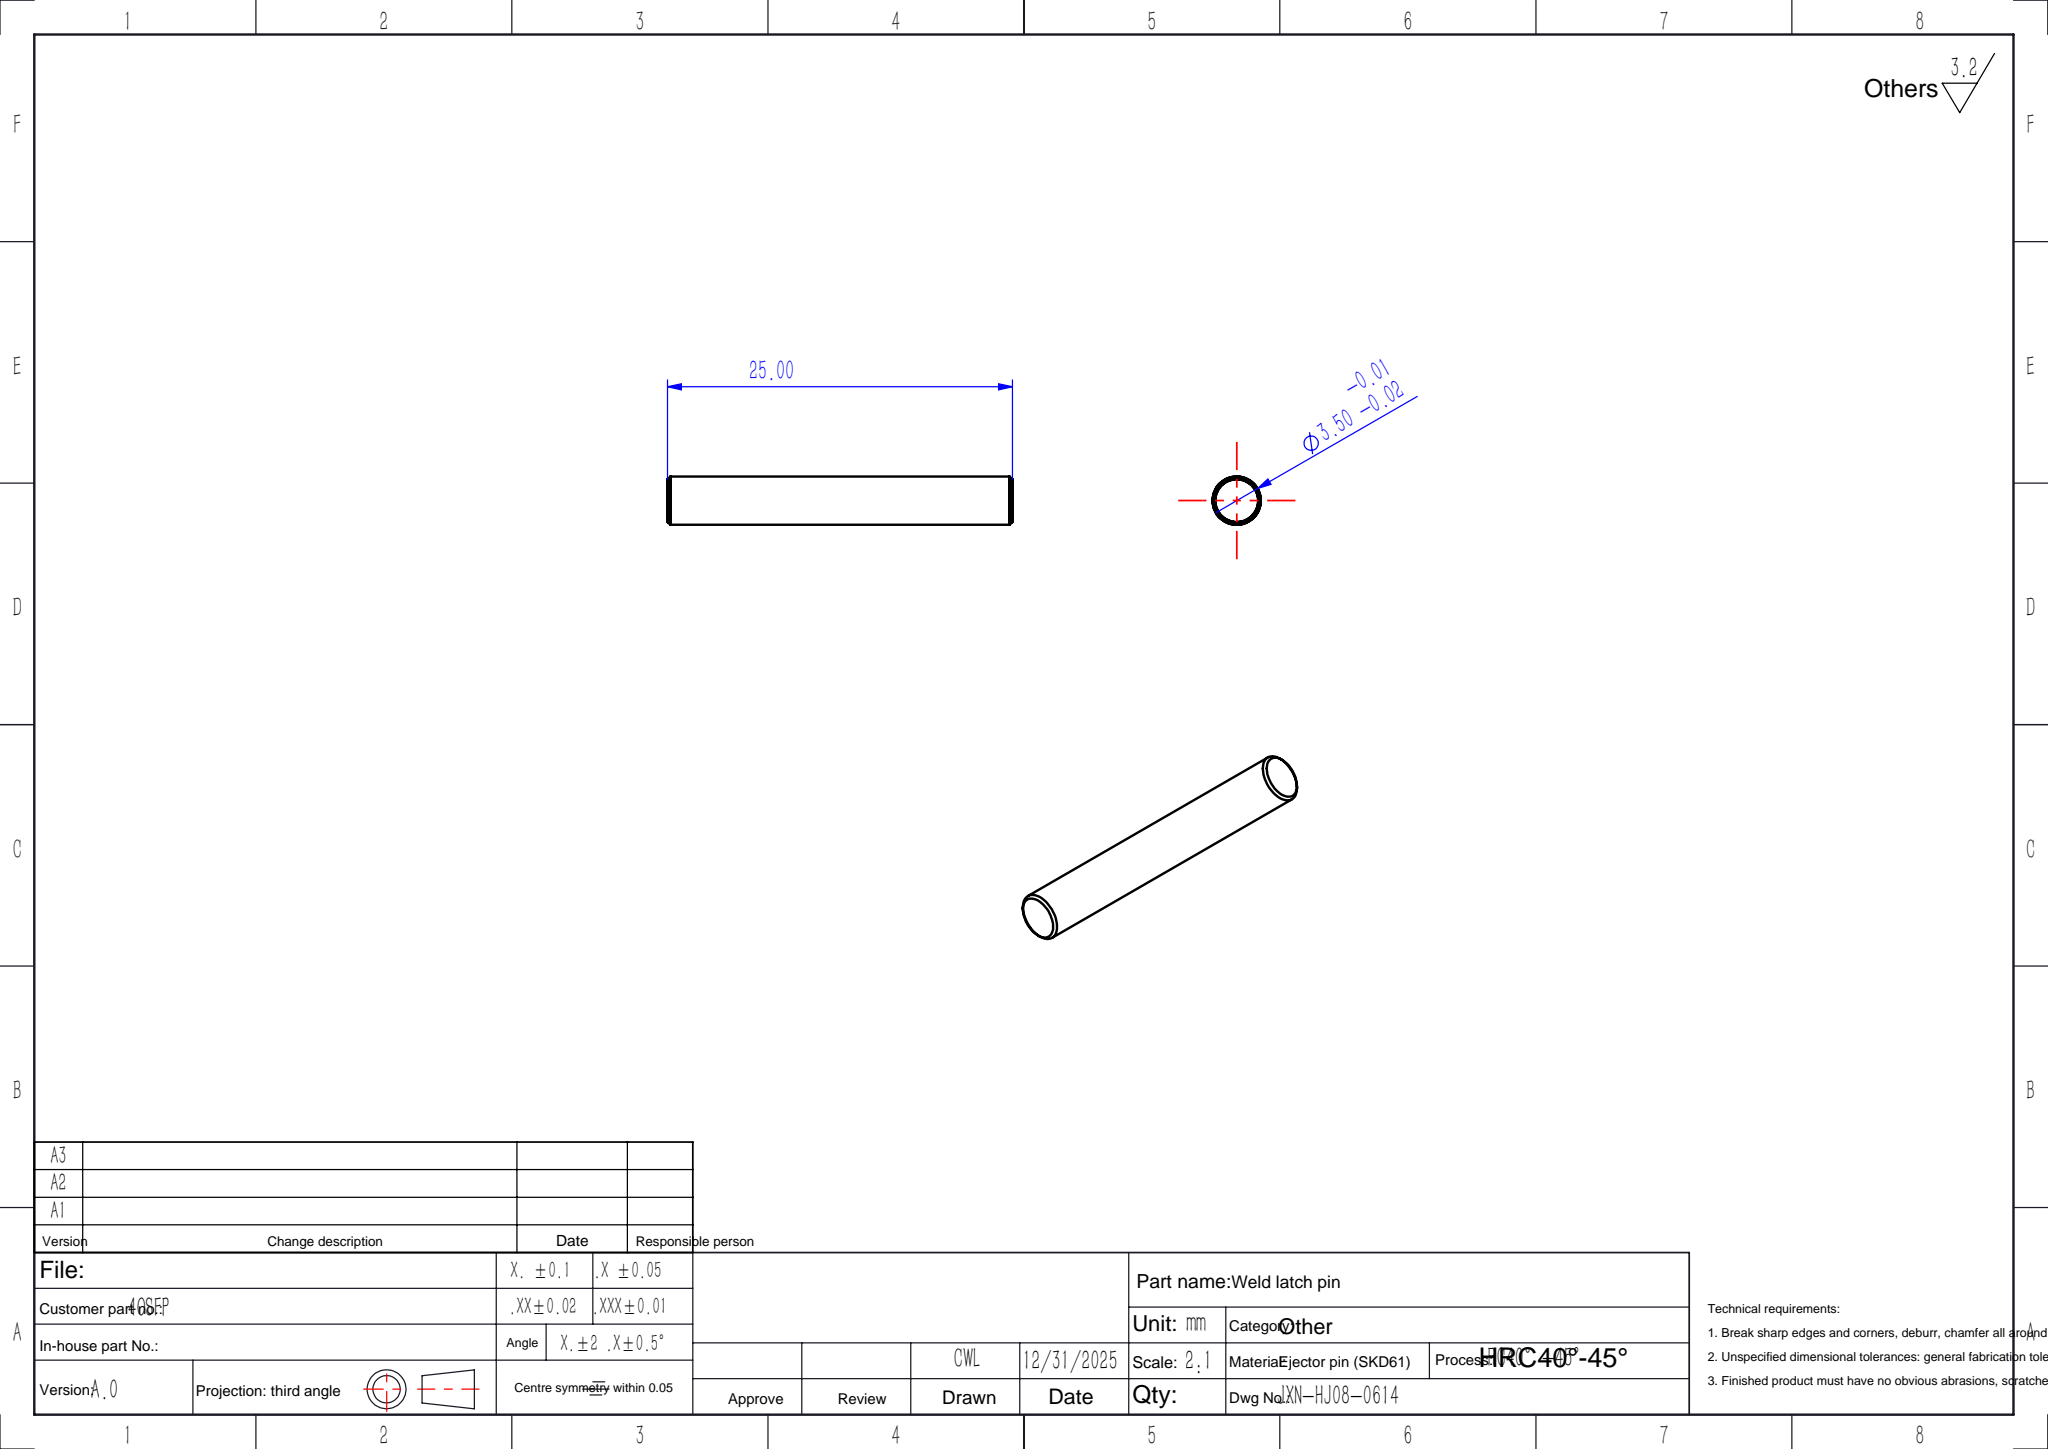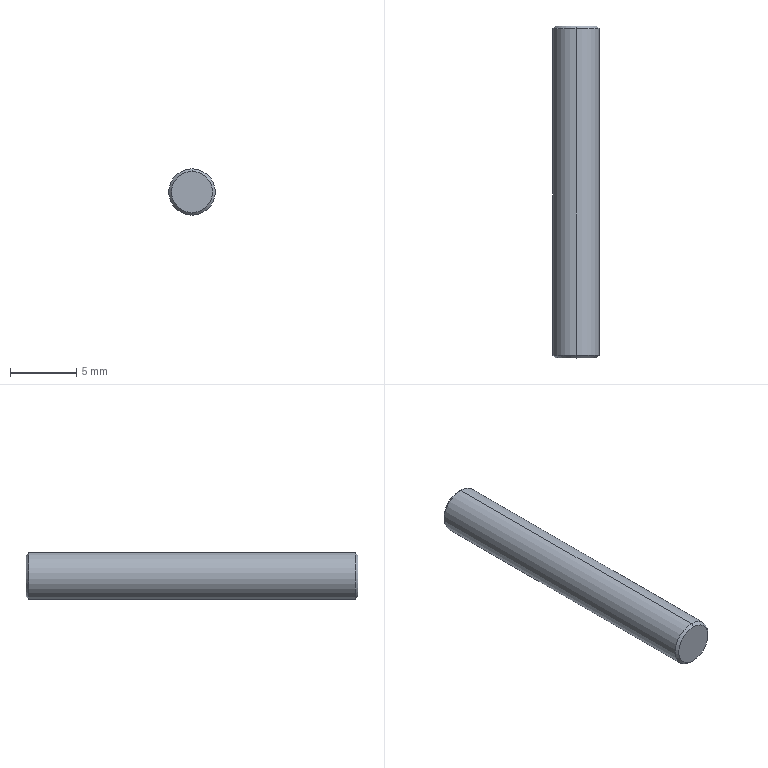Part | SolidWorks | features Chamfer 1, Extrusion 1 | 1 solid | 8 faces | box 3.5 x 25 x 3.5 mm | volume 240.105 mm3 | cone 4 | cylinder 2 | plane 2 | commonest cylinder face diameters 3.5 x2
STEP:
#1=CARTESIAN_POINT('',(0.,0.,-1.55));
#2=VERTEX_POINT('',#1);
#3=CARTESIAN_POINT('',(0.,0.,1.55));
#4=VERTEX_POINT('',#3);
#5=CARTESIAN_POINT('',(0.,0.,0.));
#6=DIRECTION('',(0.,-1.,0.));
#7=DIRECTION('',(0.,0.,1.));
#8=AXIS2_PLACEMENT_3D('',#5,#6,#7);
#9=CIRCLE('',#8,1.55);
#10=EDGE_CURVE('',#2,#4,#9,.T.);
#11=ORIENTED_EDGE('',*,*,#10,.F.);
#12=CARTESIAN_POINT('',(0.,0.2,-1.75));
#13=VERTEX_POINT('',#12);
#14=CARTESIAN_POINT('',(0.,0.2,-1.75));
#15=DIRECTION('',(0.,0.7071,-0.7071));
#16=VECTOR('',#15,1000.);
#17=LINE('',#14,#16);
#18=EDGE_CURVE('',#2,#13,#17,.T.);
#19=ORIENTED_EDGE('',*,*,#18,.T.);
#20=CARTESIAN_POINT('',(0.,0.2,1.75));
#21=VERTEX_POINT('',#20);
#22=CARTESIAN_POINT('',(0.,0.2,0.));
#23=DIRECTION('',(0.,1.,0.));
#24=DIRECTION('',(0.,0.,1.));
#25=AXIS2_PLACEMENT_3D('',#22,#23,#24);
#26=CIRCLE('',#25,1.75);
#27=EDGE_CURVE('',#21,#13,#26,.T.);
#28=ORIENTED_EDGE('',*,*,#27,.F.);
#29=CARTESIAN_POINT('',(0.,0.2,1.75));
#30=DIRECTION('',(0.,0.7071,0.7071));
#31=VECTOR('',#30,1000.);
#32=LINE('',#29,#31);
#33=EDGE_CURVE('',#4,#21,#32,.T.);
#34=ORIENTED_EDGE('',*,*,#33,.F.);
#35=EDGE_LOOP('',(#11,#19,#28,#34));
#36=FACE_OUTER_BOUND('',#35,.T.);
#37=CARTESIAN_POINT('',(0.,0.2,0.));
#38=DIRECTION('',(0.,1.,0.));
#39=DIRECTION('',(0.,0.,1.));
#40=AXIS2_PLACEMENT_3D('',#37,#38,#39);
#41=CONICAL_SURFACE('',#40,1.75,0.7854);
#42=ADVANCED_FACE('',(#36),#41,.T.);
#43=CARTESIAN_POINT('',(0.,25.,1.55));
#44=VERTEX_POINT('',#43);
#45=CARTESIAN_POINT('',(0.,25.,-1.55));
#46=VERTEX_POINT('',#45);
#47=CARTESIAN_POINT('',(0.,25.,0.));
#48=DIRECTION('',(0.,1.,0.));
#49=DIRECTION('',(0.,0.,1.));
#50=AXIS2_PLACEMENT_3D('',#47,#48,#49);
#51=CIRCLE('',#50,1.55);
#52=EDGE_CURVE('',#44,#46,#51,.T.);
#53=ORIENTED_EDGE('',*,*,#52,.F.);
#54=CARTESIAN_POINT('',(0.,24.8,1.75));
#55=VERTEX_POINT('',#54);
#56=CARTESIAN_POINT('',(0.,25.,1.55));
#57=DIRECTION('',(0.,-0.7071,0.7071));
#58=VECTOR('',#57,1000.);
#59=LINE('',#56,#58);
#60=EDGE_CURVE('',#44,#55,#59,.T.);
#61=ORIENTED_EDGE('',*,*,#60,.T.);
#62=CARTESIAN_POINT('',(0.,24.8,-1.75));
#63=VERTEX_POINT('',#62);
#64=CARTESIAN_POINT('',(0.,24.8,0.));
#65=DIRECTION('',(0.,-1.,0.));
#66=DIRECTION('',(0.,0.,1.));
#67=AXIS2_PLACEMENT_3D('',#64,#65,#66);
#68=CIRCLE('',#67,1.75);
#69=EDGE_CURVE('',#63,#55,#68,.T.);
#70=ORIENTED_EDGE('',*,*,#69,.F.);
#71=CARTESIAN_POINT('',(0.,25.,-1.55));
#72=DIRECTION('',(0.,-0.7071,-0.7071));
#73=VECTOR('',#72,1000.);
#74=LINE('',#71,#73);
#75=EDGE_CURVE('',#46,#63,#74,.T.);
#76=ORIENTED_EDGE('',*,*,#75,.F.);
#77=EDGE_LOOP('',(#53,#61,#70,#76));
#78=FACE_OUTER_BOUND('',#77,.T.);
#79=CARTESIAN_POINT('',(0.,25.,0.));
#80=DIRECTION('',(0.,-1.,0.));
#81=DIRECTION('',(0.,0.,-1.));
#82=AXIS2_PLACEMENT_3D('',#79,#80,#81);
#83=CONICAL_SURFACE('',#82,1.55,0.7854);
#84=ADVANCED_FACE('',(#78),#83,.T.);
#85=ORIENTED_EDGE('',*,*,#69,.T.);
#86=CARTESIAN_POINT('',(0.,25.,1.75));
#87=DIRECTION('',(0.,-1.,0.));
#88=VECTOR('',#87,1000.);
#89=LINE('',#86,#88);
#90=EDGE_CURVE('',#55,#21,#89,.T.);
#91=ORIENTED_EDGE('',*,*,#90,.T.);
#92=ORIENTED_EDGE('',*,*,#27,.T.);
#93=CARTESIAN_POINT('',(0.,25.,-1.75));
#94=DIRECTION('',(0.,-1.,0.));
#95=VECTOR('',#94,1000.);
#96=LINE('',#93,#95);
#97=EDGE_CURVE('',#63,#13,#96,.T.);
#98=ORIENTED_EDGE('',*,*,#97,.F.);
#99=EDGE_LOOP('',(#85,#91,#92,#98));
#100=FACE_OUTER_BOUND('',#99,.T.);
#101=CARTESIAN_POINT('',(0.,25.,0.));
#102=DIRECTION('',(0.,-1.,0.));
#103=DIRECTION('',(0.,0.,-1.));
#104=AXIS2_PLACEMENT_3D('',#101,#102,#103);
#105=CYLINDRICAL_SURFACE('',#104,1.75);
#106=ADVANCED_FACE('',(#100),#105,.T.);
#107=ORIENTED_EDGE('',*,*,#90,.F.);
#108=CARTESIAN_POINT('',(0.,24.8,0.));
#109=DIRECTION('',(0.,-1.,0.));
#110=DIRECTION('',(0.,0.,1.));
#111=AXIS2_PLACEMENT_3D('',#108,#109,#110);
#112=CIRCLE('',#111,1.75);
#113=EDGE_CURVE('',#55,#63,#112,.T.);
#114=ORIENTED_EDGE('',*,*,#113,.T.);
#115=ORIENTED_EDGE('',*,*,#97,.T.);
#116=CARTESIAN_POINT('',(0.,0.2,0.));
#117=DIRECTION('',(0.,1.,0.));
#118=DIRECTION('',(0.,0.,1.));
#119=AXIS2_PLACEMENT_3D('',#116,#117,#118);
#120=CIRCLE('',#119,1.75);
#121=EDGE_CURVE('',#13,#21,#120,.T.);
#122=ORIENTED_EDGE('',*,*,#121,.T.);
#123=EDGE_LOOP('',(#107,#114,#115,#122));
#124=FACE_OUTER_BOUND('',#123,.T.);
#125=CARTESIAN_POINT('',(0.,25.,0.));
#126=DIRECTION('',(0.,-1.,0.));
#127=DIRECTION('',(0.,0.,-1.));
#128=AXIS2_PLACEMENT_3D('',#125,#126,#127);
#129=CYLINDRICAL_SURFACE('',#128,1.75);
#130=ADVANCED_FACE('',(#124),#129,.T.);
#131=CARTESIAN_POINT('',(0.,25.,0.));
#132=DIRECTION('',(0.,1.,0.));
#133=DIRECTION('',(0.,0.,1.));
#134=AXIS2_PLACEMENT_3D('',#131,#132,#133);
#135=CIRCLE('',#134,1.55);
#136=EDGE_CURVE('',#46,#44,#135,.T.);
#137=ORIENTED_EDGE('',*,*,#136,.T.);
#138=ORIENTED_EDGE('',*,*,#52,.T.);
#139=EDGE_LOOP('',(#137,#138));
#140=FACE_OUTER_BOUND('',#139,.T.);
#141=CARTESIAN_POINT('',(0.,25.,0.));
#142=DIRECTION('',(0.,1.,0.));
#143=DIRECTION('',(0.,0.,1.));
#144=AXIS2_PLACEMENT_3D('',#141,#142,#143);
#145=PLANE('',#144);
#146=ADVANCED_FACE('',(#140),#145,.T.);
#147=CARTESIAN_POINT('',(0.,0.,0.));
#148=DIRECTION('',(0.,-1.,0.));
#149=DIRECTION('',(0.,0.,1.));
#150=AXIS2_PLACEMENT_3D('',#147,#148,#149);
#151=CIRCLE('',#150,1.55);
#152=EDGE_CURVE('',#4,#2,#151,.T.);
#153=ORIENTED_EDGE('',*,*,#152,.T.);
#154=ORIENTED_EDGE('',*,*,#10,.T.);
#155=EDGE_LOOP('',(#153,#154));
#156=FACE_OUTER_BOUND('',#155,.T.);
#157=CARTESIAN_POINT('',(0.,0.,0.));
#158=DIRECTION('',(0.,1.,0.));
#159=DIRECTION('',(0.,0.,1.));
#160=AXIS2_PLACEMENT_3D('',#157,#158,#159);
#161=PLANE('',#160);
#162=ADVANCED_FACE('',(#156),#161,.F.);
#163=ORIENTED_EDGE('',*,*,#60,.F.);
#164=ORIENTED_EDGE('',*,*,#136,.F.);
#165=ORIENTED_EDGE('',*,*,#75,.T.);
#166=ORIENTED_EDGE('',*,*,#113,.F.);
#167=EDGE_LOOP('',(#163,#164,#165,#166));
#168=FACE_OUTER_BOUND('',#167,.T.);
#169=CARTESIAN_POINT('',(0.,25.,0.));
#170=DIRECTION('',(0.,-1.,0.));
#171=DIRECTION('',(0.,0.,-1.));
#172=AXIS2_PLACEMENT_3D('',#169,#170,#171);
#173=CONICAL_SURFACE('',#172,1.55,0.7854);
#174=ADVANCED_FACE('',(#168),#173,.T.);
#175=ORIENTED_EDGE('',*,*,#18,.F.);
#176=ORIENTED_EDGE('',*,*,#152,.F.);
#177=ORIENTED_EDGE('',*,*,#33,.T.);
#178=ORIENTED_EDGE('',*,*,#121,.F.);
#179=EDGE_LOOP('',(#175,#176,#177,#178));
#180=FACE_OUTER_BOUND('',#179,.T.);
#181=CARTESIAN_POINT('',(0.,0.2,0.));
#182=DIRECTION('',(0.,1.,0.));
#183=DIRECTION('',(0.,0.,1.));
#184=AXIS2_PLACEMENT_3D('',#181,#182,#183);
#185=CONICAL_SURFACE('',#184,1.75,0.7854);
#186=ADVANCED_FACE('',(#180),#185,.T.);
#187=CLOSED_SHELL('',(#42,#84,#106,#130,#146,#162,#174,#186));
#188=MANIFOLD_SOLID_BREP('',#187);
#189=CARTESIAN_POINT('',(0.,0.,0.));
#190=DIRECTION('',(0.,0.,1.));
#191=DIRECTION('',(1.,0.,0.));
#192=AXIS2_PLACEMENT_3D('',#189,#190,#191);
#193=(LENGTH_UNIT()NAMED_UNIT(*)SI_UNIT(.MILLI.,.METRE.));
#194=UNCERTAINTY_MEASURE_WITH_UNIT(LENGTH_MEASURE(0.00001),#193,'','');
#195=(NAMED_UNIT(*)PLANE_ANGLE_UNIT()SI_UNIT($,.RADIAN.));
#196=(NAMED_UNIT(*)SI_UNIT($,.STERADIAN.)SOLID_ANGLE_UNIT());
#197=(GEOMETRIC_REPRESENTATION_CONTEXT(3)GLOBAL_UNCERTAINTY_ASSIGNED_CONTEXT((#194))GLOBAL_UNIT_ASSIGNED_CONTEXT((#193,#195,#196))REPRESENTATION_CONTEXT('',''));
#198=ADVANCED_BREP_SHAPE_REPRESENTATION('',(#188,#192),#197);